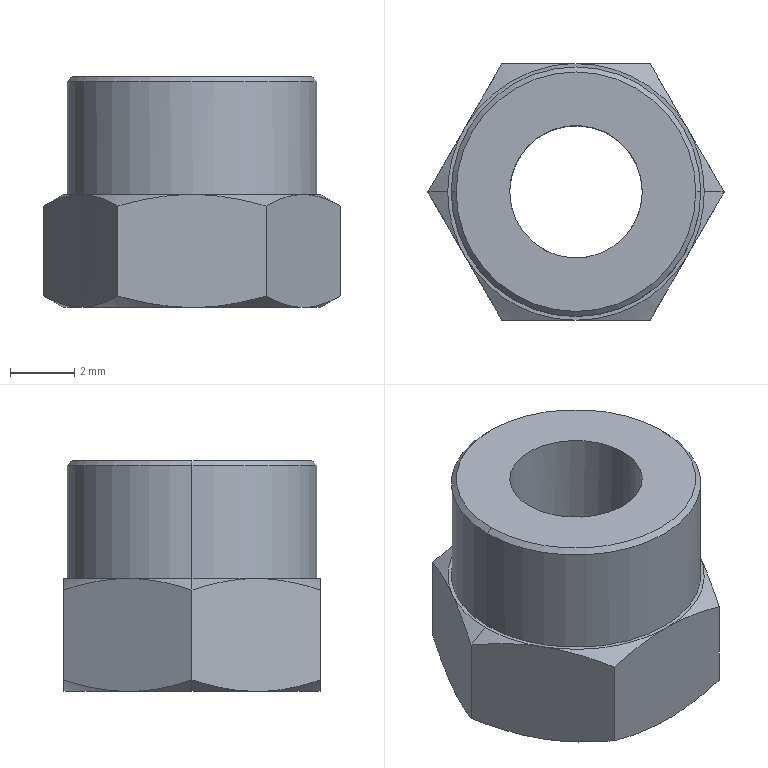Part | STEP file | 46A-01001LM15_Default<As Machined> | 1 solid | 73 faces | box 9.238 x 8 x 7.2 mm | volume 261.678 mm3 | cone 48 | cylinder 16 | plane 9 | commonest cylinder face diameters 4.134 x14 7.78 x2